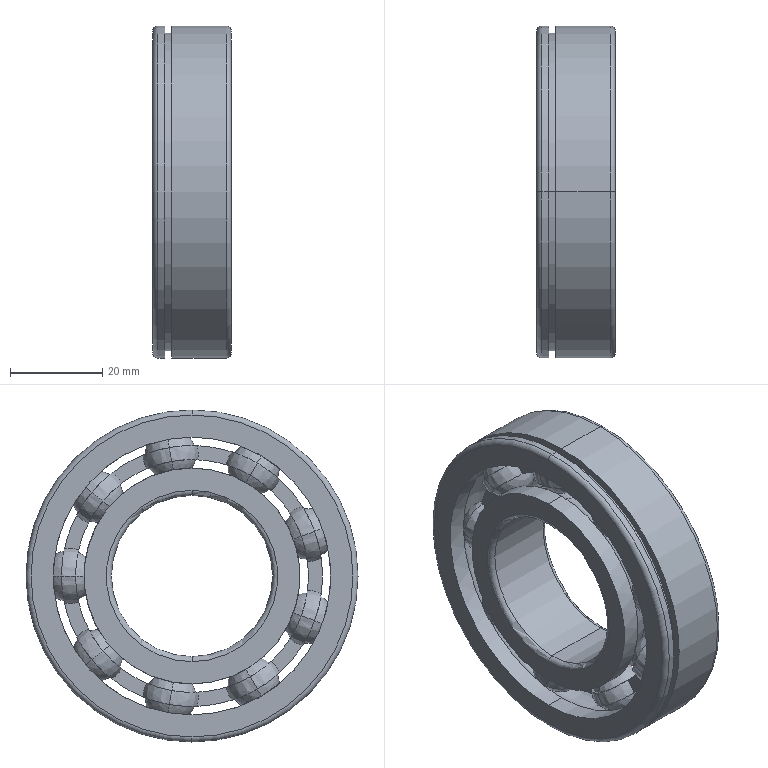Part | STEP file | GB/T276-94 deep groove ball bearing 6207-N | 1 solid | 154 faces | box 17 x 72 x 72 mm | volume 35893 mm3 | sphere 72 | torus 38 | plane 24 | cylinder 20 | commonest cylinder face diameters 46.8 x4 60.2 x4 72 x4 35 x2 50.444 x2 56.556 x2